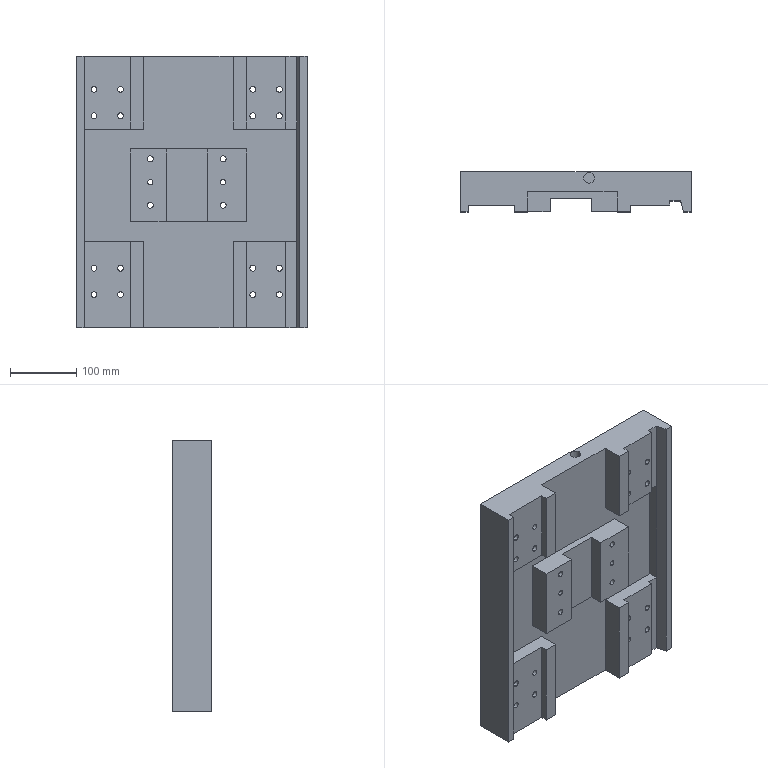Part | STEP file | Turret Tool Holder Base Plate | 1 solid | 151 faces | box 348 x 60 x 410 mm | volume 5898347 mm3 | cylinder 86 | plane 65 | commonest cylinder face diameters 9 x40 15 x40 8 x4 16 x2